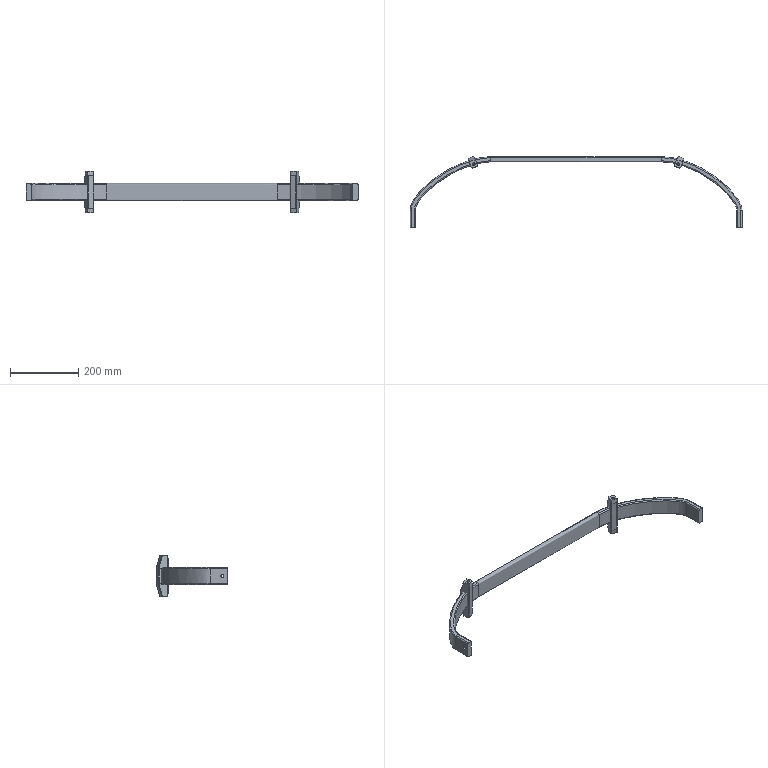Part | SolidWorks | features BaseBody 3 | 3 solids | 76 faces | box 975.001 x 207.773 x 122 mm | volume 978767 mm3 | plane 46 | spline 18 | cylinder 12 | commonest cylinder face diameters 6 x4 7.765 x4 8 x4